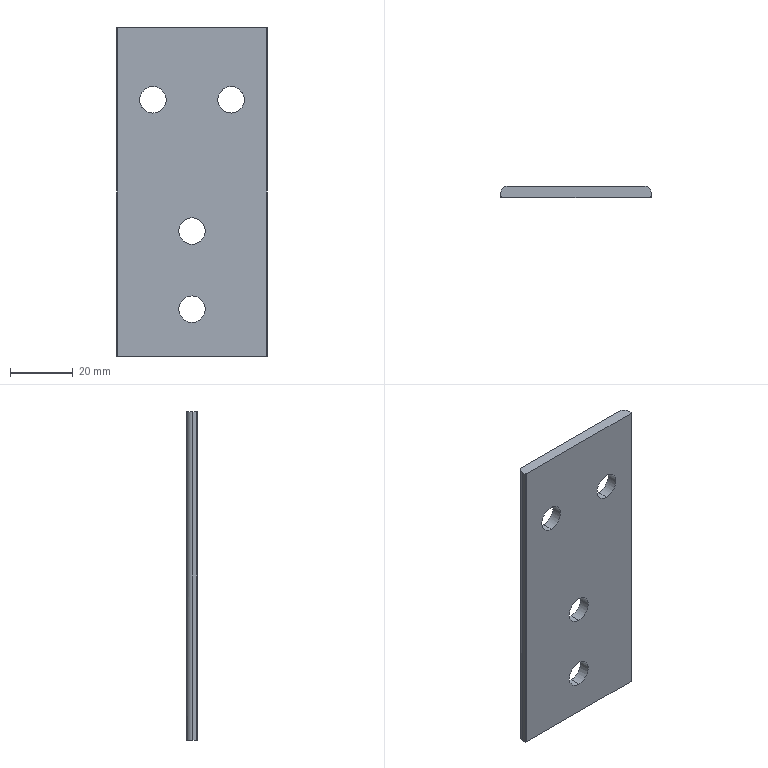Part | STEP file | 31E-01025QY13 | 1 solid | 18 faces | box 48 x 3.5 x 105 mm | volume 16661 mm3 | cylinder 12 | plane 6 | commonest cylinder face diameters 8.5 x8 0.6 x2 4 x2
STEP:
#1=CARTESIAN_POINT('',(0.,-1.75,10.75));
#2=VERTEX_POINT('',#1);
#3=CARTESIAN_POINT('',(0.,-1.75,19.25));
#4=VERTEX_POINT('',#3);
#5=CARTESIAN_POINT('',(0.,-1.75,15.));
#6=DIRECTION('',(0.,1.,0.));
#7=AXIS2_PLACEMENT_3D('',#5,#6,$);
#8=CIRCLE('',#7,4.25);
#9=EDGE_CURVE('',#2,#4,#8,.T.);
#10=ORIENTED_EDGE('',*,*,#9,.F.);
#11=CARTESIAN_POINT('',(0.,1.75,10.75));
#12=VERTEX_POINT('',#11);
#13=CARTESIAN_POINT('',(0.,-1.75,10.75));
#14=DIRECTION('',(0.,1.,0.));
#15=VECTOR('',#14,1.);
#16=LINE('',#13,#15);
#17=EDGE_CURVE('',#2,#12,#16,.T.);
#18=ORIENTED_EDGE('',*,*,#17,.T.);
#19=CARTESIAN_POINT('',(0.,1.75,19.25));
#20=VERTEX_POINT('',#19);
#21=CARTESIAN_POINT('',(0.,1.75,15.));
#22=DIRECTION('',(0.,1.,0.));
#23=AXIS2_PLACEMENT_3D('',#21,#22,$);
#24=CIRCLE('',#23,4.25);
#25=EDGE_CURVE('',#12,#20,#24,.T.);
#26=ORIENTED_EDGE('',*,*,#25,.T.);
#27=CARTESIAN_POINT('',(0.,-1.75,19.25));
#28=DIRECTION('',(0.,1.,0.));
#29=VECTOR('',#28,1.);
#30=LINE('',#27,#29);
#31=EDGE_CURVE('',#4,#20,#30,.T.);
#32=ORIENTED_EDGE('',*,*,#31,.F.);
#33=EDGE_LOOP('',(#10,#18,#26,#32));
#34=FACE_OUTER_BOUND('',#33,.T.);
#35=CARTESIAN_POINT('',(0.,-1.75,15.));
#36=DIRECTION('',(0.,1.,0.));
#37=DIRECTION('',(0.,0.,-1.));
#38=AXIS2_PLACEMENT_3D('',#35,#36,#37);
#39=CYLINDRICAL_SURFACE('',#38,4.25);
#40=ADVANCED_FACE('',(#34),#39,.F.);
#41=CARTESIAN_POINT('',(-23.7,-1.75,105.));
#42=VERTEX_POINT('',#41);
#43=CARTESIAN_POINT('',(23.7,-1.75,105.));
#44=VERTEX_POINT('',#43);
#45=CARTESIAN_POINT('',(0.,-1.75,105.));
#46=DIRECTION('',(1.,0.,0.));
#47=VECTOR('',#46,1.);
#48=LINE('',#45,#47);
#49=EDGE_CURVE('',#42,#44,#48,.T.);
#50=ORIENTED_EDGE('',*,*,#49,.F.);
#51=CARTESIAN_POINT('',(-23.7,-1.75,0.));
#52=VERTEX_POINT('',#51);
#53=CARTESIAN_POINT('',(-23.7,-1.75,52.5));
#54=DIRECTION('',(0.,0.,-1.));
#55=VECTOR('',#54,1.);
#56=LINE('',#53,#55);
#57=EDGE_CURVE('',#42,#52,#56,.T.);
#58=ORIENTED_EDGE('',*,*,#57,.T.);
#59=CARTESIAN_POINT('',(23.7,-1.75,0.));
#60=VERTEX_POINT('',#59);
#61=CARTESIAN_POINT('',(0.,-1.75,0.));
#62=DIRECTION('',(1.,0.,0.));
#63=VECTOR('',#62,1.);
#64=LINE('',#61,#63);
#65=EDGE_CURVE('',#52,#60,#64,.T.);
#66=ORIENTED_EDGE('',*,*,#65,.T.);
#67=CARTESIAN_POINT('',(23.7,-1.75,52.5));
#68=DIRECTION('',(0.,0.,1.));
#69=VECTOR('',#68,1.);
#70=LINE('',#67,#69);
#71=EDGE_CURVE('',#60,#44,#70,.T.);
#72=ORIENTED_EDGE('',*,*,#71,.T.);
#73=EDGE_LOOP('',(#50,#58,#66,#72));
#74=FACE_OUTER_BOUND('',#73,.T.);
#75=CARTESIAN_POINT('',(0.,-1.75,15.));
#76=DIRECTION('',(0.,1.,0.));
#77=AXIS2_PLACEMENT_3D('',#75,#76,$);
#78=CIRCLE('',#77,4.25);
#79=EDGE_CURVE('',#4,#2,#78,.T.);
#80=ORIENTED_EDGE('',*,*,#79,.T.);
#81=ORIENTED_EDGE('',*,*,#9,.T.);
#82=EDGE_LOOP('',(#80,#81));
#83=FACE_BOUND('',#82,.T.);
#84=CARTESIAN_POINT('',(0.,-1.75,44.25));
#85=VERTEX_POINT('',#84);
#86=CARTESIAN_POINT('',(0.,-1.75,35.75));
#87=VERTEX_POINT('',#86);
#88=CARTESIAN_POINT('',(0.,-1.75,40.));
#89=DIRECTION('',(0.,1.,0.));
#90=AXIS2_PLACEMENT_3D('',#88,#89,$);
#91=CIRCLE('',#90,4.25);
#92=EDGE_CURVE('',#85,#87,#91,.T.);
#93=ORIENTED_EDGE('',*,*,#92,.T.);
#94=CARTESIAN_POINT('',(0.,-1.75,40.));
#95=DIRECTION('',(0.,1.,0.));
#96=AXIS2_PLACEMENT_3D('',#94,#95,$);
#97=CIRCLE('',#96,4.25);
#98=EDGE_CURVE('',#87,#85,#97,.T.);
#99=ORIENTED_EDGE('',*,*,#98,.T.);
#100=EDGE_LOOP('',(#93,#99));
#101=FACE_BOUND('',#100,.T.);
#102=CARTESIAN_POINT('',(12.5,-1.75,86.25));
#103=VERTEX_POINT('',#102);
#104=CARTESIAN_POINT('',(12.5,-1.75,77.75));
#105=VERTEX_POINT('',#104);
#106=CARTESIAN_POINT('',(12.5,-1.75,82.));
#107=DIRECTION('',(0.,1.,0.));
#108=AXIS2_PLACEMENT_3D('',#106,#107,$);
#109=CIRCLE('',#108,4.25);
#110=EDGE_CURVE('',#103,#105,#109,.T.);
#111=ORIENTED_EDGE('',*,*,#110,.T.);
#112=CARTESIAN_POINT('',(12.5,-1.75,82.));
#113=DIRECTION('',(0.,1.,0.));
#114=AXIS2_PLACEMENT_3D('',#112,#113,$);
#115=CIRCLE('',#114,4.25);
#116=EDGE_CURVE('',#105,#103,#115,.T.);
#117=ORIENTED_EDGE('',*,*,#116,.T.);
#118=EDGE_LOOP('',(#111,#117));
#119=FACE_BOUND('',#118,.T.);
#120=CARTESIAN_POINT('',(-12.5,-1.75,86.25));
#121=VERTEX_POINT('',#120);
#122=CARTESIAN_POINT('',(-12.5,-1.75,77.75));
#123=VERTEX_POINT('',#122);
#124=CARTESIAN_POINT('',(-12.5,-1.75,82.));
#125=DIRECTION('',(0.,1.,0.));
#126=AXIS2_PLACEMENT_3D('',#124,#125,$);
#127=CIRCLE('',#126,4.25);
#128=EDGE_CURVE('',#121,#123,#127,.T.);
#129=ORIENTED_EDGE('',*,*,#128,.T.);
#130=CARTESIAN_POINT('',(-12.5,-1.75,82.));
#131=DIRECTION('',(0.,1.,0.));
#132=AXIS2_PLACEMENT_3D('',#130,#131,$);
#133=CIRCLE('',#132,4.25);
#134=EDGE_CURVE('',#123,#121,#133,.T.);
#135=ORIENTED_EDGE('',*,*,#134,.T.);
#136=EDGE_LOOP('',(#129,#135));
#137=FACE_BOUND('',#136,.T.);
#138=CARTESIAN_POINT('',(-24.,-1.75,105.));
#139=DIRECTION('',(0.,1.,0.));
#140=DIRECTION('',(0.,0.,1.));
#141=AXIS2_PLACEMENT_3D('',#138,#139,#140);
#142=PLANE('',#141);
#143=ADVANCED_FACE('',(#74,#83,#101,#119,#137),#142,.F.);
#144=ORIENTED_EDGE('',*,*,#17,.F.);
#145=ORIENTED_EDGE('',*,*,#79,.F.);
#146=ORIENTED_EDGE('',*,*,#31,.T.);
#147=CARTESIAN_POINT('',(0.,1.75,15.));
#148=DIRECTION('',(0.,1.,0.));
#149=AXIS2_PLACEMENT_3D('',#147,#148,$);
#150=CIRCLE('',#149,4.25);
#151=EDGE_CURVE('',#20,#12,#150,.T.);
#152=ORIENTED_EDGE('',*,*,#151,.T.);
#153=EDGE_LOOP('',(#144,#145,#146,#152));
#154=FACE_OUTER_BOUND('',#153,.T.);
#155=CARTESIAN_POINT('',(0.,-1.75,15.));
#156=DIRECTION('',(0.,1.,0.));
#157=DIRECTION('',(0.,0.,1.));
#158=AXIS2_PLACEMENT_3D('',#155,#156,#157);
#159=CYLINDRICAL_SURFACE('',#158,4.25);
#160=ADVANCED_FACE('',(#154),#159,.F.);
#161=CARTESIAN_POINT('',(22.,1.75,0.));
#162=VERTEX_POINT('',#161);
#163=CARTESIAN_POINT('',(-22.,1.75,0.));
#164=VERTEX_POINT('',#163);
#165=CARTESIAN_POINT('',(0.,1.75,0.));
#166=DIRECTION('',(-1.,0.,0.));
#167=VECTOR('',#166,1.);
#168=LINE('',#165,#167);
#169=EDGE_CURVE('',#162,#164,#168,.T.);
#170=ORIENTED_EDGE('',*,*,#169,.T.);
#171=CARTESIAN_POINT('',(-22.,1.75,105.));
#172=VERTEX_POINT('',#171);
#173=CARTESIAN_POINT('',(-22.,1.75,52.5));
#174=DIRECTION('',(0.,0.,1.));
#175=VECTOR('',#174,1.);
#176=LINE('',#173,#175);
#177=EDGE_CURVE('',#164,#172,#176,.T.);
#178=ORIENTED_EDGE('',*,*,#177,.T.);
#179=CARTESIAN_POINT('',(22.,1.75,105.));
#180=VERTEX_POINT('',#179);
#181=CARTESIAN_POINT('',(0.,1.75,105.));
#182=DIRECTION('',(-1.,0.,0.));
#183=VECTOR('',#182,1.);
#184=LINE('',#181,#183);
#185=EDGE_CURVE('',#180,#172,#184,.T.);
#186=ORIENTED_EDGE('',*,*,#185,.F.);
#187=CARTESIAN_POINT('',(22.,1.75,52.5));
#188=DIRECTION('',(0.,0.,-1.));
#189=VECTOR('',#188,1.);
#190=LINE('',#187,#189);
#191=EDGE_CURVE('',#180,#162,#190,.T.);
#192=ORIENTED_EDGE('',*,*,#191,.T.);
#193=EDGE_LOOP('',(#170,#178,#186,#192));
#194=FACE_OUTER_BOUND('',#193,.T.);
#195=ORIENTED_EDGE('',*,*,#151,.F.);
#196=ORIENTED_EDGE('',*,*,#25,.F.);
#197=EDGE_LOOP('',(#195,#196));
#198=FACE_BOUND('',#197,.T.);
#199=CARTESIAN_POINT('',(0.,1.75,44.25));
#200=VERTEX_POINT('',#199);
#201=CARTESIAN_POINT('',(0.,1.75,35.75));
#202=VERTEX_POINT('',#201);
#203=CARTESIAN_POINT('',(0.,1.75,44.25));
#204=CARTESIAN_POINT('',(0.404,1.75,44.25));
#205=CARTESIAN_POINT('',(0.808,1.75,44.202));
#206=CARTESIAN_POINT('',(1.204,1.75,44.106));
#207=CARTESIAN_POINT('',(1.967,1.75,43.822));
#208=CARTESIAN_POINT('',(2.641,1.75,43.367));
#209=CARTESIAN_POINT('',(2.95,1.75,43.1));
#210=CARTESIAN_POINT('',(3.497,1.75,42.498));
#211=CARTESIAN_POINT('',(3.889,1.75,41.785));
#212=CARTESIAN_POINT('',(4.041,1.75,41.407));
#213=CARTESIAN_POINT('',(4.253,1.75,40.621));
#214=CARTESIAN_POINT('',(4.275,1.75,39.808));
#215=CARTESIAN_POINT('',(4.237,1.75,39.402));
#216=CARTESIAN_POINT('',(4.066,1.75,38.606));
#217=CARTESIAN_POINT('',(3.713,1.75,37.873));
#218=CARTESIAN_POINT('',(3.493,1.75,37.529));
#219=CARTESIAN_POINT('',(2.977,1.75,36.9));
#220=CARTESIAN_POINT('',(2.328,1.75,36.41));
#221=CARTESIAN_POINT('',(1.976,1.75,36.204));
#222=CARTESIAN_POINT('',(1.374,1.75,35.944));
#223=CARTESIAN_POINT('',(0.7377,1.75,35.804));
#224=CARTESIAN_POINT('',(0.4929,1.75,35.768));
#225=CARTESIAN_POINT('',(0.2465,1.75,35.75));
#226=CARTESIAN_POINT('',(0.,1.75,35.75));
#227=B_SPLINE_CURVE_WITH_KNOTS('',5,(#203,#204,#205,#206,#207,#208,#209,#210,#211,#212,#213,#214,#215,#216,#217,#218,#219,#220,#221,#222,#223,#224,#225,#226),.UNSPECIFIED.,.F.,.U.,(6,3,3,3,3,3,3,6),(0.,2.857,5.713,8.57,11.426,14.283,17.139,18.882),.UNSPECIFIED.);
#228=EDGE_CURVE('',#200,#202,#227,.T.);
#229=ORIENTED_EDGE('',*,*,#228,.F.);
#230=CARTESIAN_POINT('',(0.,1.75,35.75));
#231=CARTESIAN_POINT('',(-0.404,1.75,35.75));
#232=CARTESIAN_POINT('',(-0.808,1.75,35.798));
#233=CARTESIAN_POINT('',(-1.204,1.75,35.894));
#234=CARTESIAN_POINT('',(-1.967,1.75,36.178));
#235=CARTESIAN_POINT('',(-2.641,1.75,36.633));
#236=CARTESIAN_POINT('',(-2.95,1.75,36.9));
#237=CARTESIAN_POINT('',(-3.497,1.75,37.502));
#238=CARTESIAN_POINT('',(-3.889,1.75,38.215));
#239=CARTESIAN_POINT('',(-4.041,1.75,38.593));
#240=CARTESIAN_POINT('',(-4.253,1.75,39.379));
#241=CARTESIAN_POINT('',(-4.275,1.75,40.192));
#242=CARTESIAN_POINT('',(-4.237,1.75,40.598));
#243=CARTESIAN_POINT('',(-4.066,1.75,41.394));
#244=CARTESIAN_POINT('',(-3.713,1.75,42.127));
#245=CARTESIAN_POINT('',(-3.493,1.75,42.471));
#246=CARTESIAN_POINT('',(-2.977,1.75,43.1));
#247=CARTESIAN_POINT('',(-2.328,1.75,43.59));
#248=CARTESIAN_POINT('',(-1.976,1.75,43.796));
#249=CARTESIAN_POINT('',(-1.374,1.75,44.056));
#250=CARTESIAN_POINT('',(-0.7377,1.75,44.196));
#251=CARTESIAN_POINT('',(-0.4929,1.75,44.232));
#252=CARTESIAN_POINT('',(-0.2465,1.75,44.25));
#253=CARTESIAN_POINT('',(0.,1.75,44.25));
#254=B_SPLINE_CURVE_WITH_KNOTS('',5,(#230,#231,#232,#233,#234,#235,#236,#237,#238,#239,#240,#241,#242,#243,#244,#245,#246,#247,#248,#249,#250,#251,#252,#253),.UNSPECIFIED.,.F.,.U.,(6,3,3,3,3,3,3,6),(0.,2.857,5.713,8.57,11.426,14.283,17.139,18.882),.UNSPECIFIED.);
#255=EDGE_CURVE('',#202,#200,#254,.T.);
#256=ORIENTED_EDGE('',*,*,#255,.F.);
#257=EDGE_LOOP('',(#229,#256));
#258=FACE_BOUND('',#257,.T.);
#259=CARTESIAN_POINT('',(12.5,1.75,86.25));
#260=VERTEX_POINT('',#259);
#261=CARTESIAN_POINT('',(12.5,1.75,77.75));
#262=VERTEX_POINT('',#261);
#263=CARTESIAN_POINT('',(12.5,1.75,86.25));
#264=CARTESIAN_POINT('',(12.904,1.75,86.25));
#265=CARTESIAN_POINT('',(13.308,1.75,86.202));
#266=CARTESIAN_POINT('',(13.704,1.75,86.106));
#267=CARTESIAN_POINT('',(14.467,1.75,85.822));
#268=CARTESIAN_POINT('',(15.141,1.75,85.367));
#269=CARTESIAN_POINT('',(15.45,1.75,85.1));
#270=CARTESIAN_POINT('',(15.997,1.75,84.498));
#271=CARTESIAN_POINT('',(16.389,1.75,83.785));
#272=CARTESIAN_POINT('',(16.541,1.75,83.407));
#273=CARTESIAN_POINT('',(16.753,1.75,82.621));
#274=CARTESIAN_POINT('',(16.775,1.75,81.808));
#275=CARTESIAN_POINT('',(16.737,1.75,81.402));
#276=CARTESIAN_POINT('',(16.566,1.75,80.606));
#277=CARTESIAN_POINT('',(16.213,1.75,79.873));
#278=CARTESIAN_POINT('',(15.993,1.75,79.529));
#279=CARTESIAN_POINT('',(15.477,1.75,78.9));
#280=CARTESIAN_POINT('',(14.828,1.75,78.41));
#281=CARTESIAN_POINT('',(14.476,1.75,78.204));
#282=CARTESIAN_POINT('',(13.874,1.75,77.944));
#283=CARTESIAN_POINT('',(13.238,1.75,77.804));
#284=CARTESIAN_POINT('',(12.993,1.75,77.768));
#285=CARTESIAN_POINT('',(12.746,1.75,77.75));
#286=CARTESIAN_POINT('',(12.5,1.75,77.75));
#287=B_SPLINE_CURVE_WITH_KNOTS('',5,(#263,#264,#265,#266,#267,#268,#269,#270,#271,#272,#273,#274,#275,#276,#277,#278,#279,#280,#281,#282,#283,#284,#285,#286),.UNSPECIFIED.,.F.,.U.,(6,3,3,3,3,3,3,6),(0.,2.857,5.713,8.57,11.426,14.283,17.139,18.882),.UNSPECIFIED.);
#288=EDGE_CURVE('',#260,#262,#287,.T.);
#289=ORIENTED_EDGE('',*,*,#288,.F.);
#290=CARTESIAN_POINT('',(12.5,1.75,77.75));
#291=CARTESIAN_POINT('',(12.096,1.75,77.75));
#292=CARTESIAN_POINT('',(11.692,1.75,77.798));
#293=CARTESIAN_POINT('',(11.296,1.75,77.894));
#294=CARTESIAN_POINT('',(10.533,1.75,78.178));
#295=CARTESIAN_POINT('',(9.859,1.75,78.633));
#296=CARTESIAN_POINT('',(9.55,1.75,78.9));
#297=CARTESIAN_POINT('',(9.003,1.75,79.502));
#298=CARTESIAN_POINT('',(8.611,1.75,80.215));
#299=CARTESIAN_POINT('',(8.459,1.75,80.593));
#300=CARTESIAN_POINT('',(8.247,1.75,81.379));
#301=CARTESIAN_POINT('',(8.225,1.75,82.192));
#302=CARTESIAN_POINT('',(8.263,1.75,82.598));
#303=CARTESIAN_POINT('',(8.434,1.75,83.394));
#304=CARTESIAN_POINT('',(8.787,1.75,84.127));
#305=CARTESIAN_POINT('',(9.007,1.75,84.471));
#306=CARTESIAN_POINT('',(9.523,1.75,85.1));
#307=CARTESIAN_POINT('',(10.172,1.75,85.59));
#308=CARTESIAN_POINT('',(10.524,1.75,85.796));
#309=CARTESIAN_POINT('',(11.126,1.75,86.056));
#310=CARTESIAN_POINT('',(11.762,1.75,86.196));
#311=CARTESIAN_POINT('',(12.007,1.75,86.232));
#312=CARTESIAN_POINT('',(12.254,1.75,86.25));
#313=CARTESIAN_POINT('',(12.5,1.75,86.25));
#314=B_SPLINE_CURVE_WITH_KNOTS('',5,(#290,#291,#292,#293,#294,#295,#296,#297,#298,#299,#300,#301,#302,#303,#304,#305,#306,#307,#308,#309,#310,#311,#312,#313),.UNSPECIFIED.,.F.,.U.,(6,3,3,3,3,3,3,6),(0.,2.857,5.713,8.57,11.426,14.283,17.139,18.882),.UNSPECIFIED.);
#315=EDGE_CURVE('',#262,#260,#314,.T.);
#316=ORIENTED_EDGE('',*,*,#315,.F.);
#317=EDGE_LOOP('',(#289,#316));
#318=FACE_BOUND('',#317,.T.);
#319=CARTESIAN_POINT('',(-12.5,1.75,86.25));
#320=VERTEX_POINT('',#319);
#321=CARTESIAN_POINT('',(-12.5,1.75,77.75));
#322=VERTEX_POINT('',#321);
#323=CARTESIAN_POINT('',(-12.5,1.75,86.25));
#324=CARTESIAN_POINT('',(-12.096,1.75,86.25));
#325=CARTESIAN_POINT('',(-11.692,1.75,86.202));
#326=CARTESIAN_POINT('',(-11.296,1.75,86.106));
#327=CARTESIAN_POINT('',(-10.533,1.75,85.822));
#328=CARTESIAN_POINT('',(-9.859,1.75,85.367));
#329=CARTESIAN_POINT('',(-9.55,1.75,85.1));
#330=CARTESIAN_POINT('',(-9.003,1.75,84.498));
#331=CARTESIAN_POINT('',(-8.611,1.75,83.785));
#332=CARTESIAN_POINT('',(-8.459,1.75,83.407));
#333=CARTESIAN_POINT('',(-8.247,1.75,82.621));
#334=CARTESIAN_POINT('',(-8.225,1.75,81.808));
#335=CARTESIAN_POINT('',(-8.263,1.75,81.402));
#336=CARTESIAN_POINT('',(-8.434,1.75,80.606));
#337=CARTESIAN_POINT('',(-8.787,1.75,79.873));
#338=CARTESIAN_POINT('',(-9.007,1.75,79.529));
#339=CARTESIAN_POINT('',(-9.523,1.75,78.9));
#340=CARTESIAN_POINT('',(-10.172,1.75,78.41));
#341=CARTESIAN_POINT('',(-10.524,1.75,78.204));
#342=CARTESIAN_POINT('',(-11.126,1.75,77.944));
#343=CARTESIAN_POINT('',(-11.762,1.75,77.804));
#344=CARTESIAN_POINT('',(-12.007,1.75,77.768));
#345=CARTESIAN_POINT('',(-12.254,1.75,77.75));
#346=CARTESIAN_POINT('',(-12.5,1.75,77.75));
#347=B_SPLINE_CURVE_WITH_KNOTS('',5,(#323,#324,#325,#326,#327,#328,#329,#330,#331,#332,#333,#334,#335,#336,#337,#338,#339,#340,#341,#342,#343,#344,#345,#346),.UNSPECIFIED.,.F.,.U.,(6,3,3,3,3,3,3,6),(0.,2.857,5.713,8.57,11.426,14.283,17.139,18.882),.UNSPECIFIED.);
#348=EDGE_CURVE('',#320,#322,#347,.T.);
#349=ORIENTED_EDGE('',*,*,#348,.F.);
#350=CARTESIAN_POINT('',(-12.5,1.75,77.75));
#351=CARTESIAN_POINT('',(-12.904,1.75,77.75));
#352=CARTESIAN_POINT('',(-13.308,1.75,77.798));
#353=CARTESIAN_POINT('',(-13.704,1.75,77.894));
#354=CARTESIAN_POINT('',(-14.467,1.75,78.178));
#355=CARTESIAN_POINT('',(-15.141,1.75,78.633));
#356=CARTESIAN_POINT('',(-15.45,1.75,78.9));
#357=CARTESIAN_POINT('',(-15.997,1.75,79.502));
#358=CARTESIAN_POINT('',(-16.389,1.75,80.215));
#359=CARTESIAN_POINT('',(-16.541,1.75,80.593));
#360=CARTESIAN_POINT('',(-16.753,1.75,81.379));
#361=CARTESIAN_POINT('',(-16.775,1.75,82.192));
#362=CARTESIAN_POINT('',(-16.737,1.75,82.598));
#363=CARTESIAN_POINT('',(-16.566,1.75,83.394));
#364=CARTESIAN_POINT('',(-16.213,1.75,84.127));
#365=CARTESIAN_POINT('',(-15.993,1.75,84.471));
#366=CARTESIAN_POINT('',(-15.477,1.75,85.1));
#367=CARTESIAN_POINT('',(-14.828,1.75,85.59));
#368=CARTESIAN_POINT('',(-14.476,1.75,85.796));
#369=CARTESIAN_POINT('',(-13.874,1.75,86.056));
#370=CARTESIAN_POINT('',(-13.238,1.75,86.196));
#371=CARTESIAN_POINT('',(-12.993,1.75,86.232));
#372=CARTESIAN_POINT('',(-12.746,1.75,86.25));
#373=CARTESIAN_POINT('',(-12.5,1.75,86.25));
#374=B_SPLINE_CURVE_WITH_KNOTS('',5,(#350,#351,#352,#353,#354,#355,#356,#357,#358,#359,#360,#361,#362,#363,#364,#365,#366,#367,#368,#369,#370,#371,#372,#373),.UNSPECIFIED.,.F.,.U.,(6,3,3,3,3,3,3,6),(0.,2.857,5.713,8.57,11.426,14.283,17.139,18.882),.UNSPECIFIED.);
#375=EDGE_CURVE('',#322,#320,#374,.T.);
#376=ORIENTED_EDGE('',*,*,#375,.F.);
#377=EDGE_LOOP('',(#349,#376));
#378=FACE_BOUND('',#377,.T.);
#379=CARTESIAN_POINT('',(-24.,1.75,105.));
#380=DIRECTION('',(0.,-1.,0.));
#381=DIRECTION('',(0.,0.,-1.));
#382=AXIS2_PLACEMENT_3D('',#379,#380,#381);
#383=PLANE('',#382);
#384=ADVANCED_FACE('',(#194,#198,#258,#318,#378),#383,.F.);
#385=CARTESIAN_POINT('',(-24.,-0.25,105.));
#386=VERTEX_POINT('',#385);
#387=CARTESIAN_POINT('',(-24.,-1.45,105.));
#388=VERTEX_POINT('',#387);
#389=CARTESIAN_POINT('',(-24.,-0.85,105.));
#390=DIRECTION('',(0.,-1.,0.));
#391=VECTOR('',#390,1.);
#392=LINE('',#389,#391);
#393=EDGE_CURVE('',#386,#388,#392,.T.);
#394=ORIENTED_EDGE('',*,*,#393,.T.);
#395=CARTESIAN_POINT('',(-23.7,-1.45,105.));
#396=DIRECTION('',(0.,0.,1.));
#397=AXIS2_PLACEMENT_3D('',#395,#396,$);
#398=CIRCLE('',#397,0.3);
#399=EDGE_CURVE('',#388,#42,#398,.T.);
#400=ORIENTED_EDGE('',*,*,#399,.T.);
#401=ORIENTED_EDGE('',*,*,#49,.T.);
#402=CARTESIAN_POINT('',(24.,-1.45,105.));
#403=VERTEX_POINT('',#402);
#404=CARTESIAN_POINT('',(23.7,-1.45,105.));
#405=DIRECTION('',(0.,0.,1.));
#406=AXIS2_PLACEMENT_3D('',#404,#405,$);
#407=CIRCLE('',#406,0.3);
#408=EDGE_CURVE('',#44,#403,#407,.T.);
#409=ORIENTED_EDGE('',*,*,#408,.T.);
#410=CARTESIAN_POINT('',(24.,-0.25,105.));
#411=VERTEX_POINT('',#410);
#412=CARTESIAN_POINT('',(24.,-0.85,105.));
#413=DIRECTION('',(0.,1.,0.));
#414=VECTOR('',#413,1.);
#415=LINE('',#412,#414);
#416=EDGE_CURVE('',#403,#411,#415,.T.);
#417=ORIENTED_EDGE('',*,*,#416,.T.);
#418=CARTESIAN_POINT('',(22.,-0.25,105.));
#419=DIRECTION('',(0.,0.,1.));
#420=AXIS2_PLACEMENT_3D('',#418,#419,$);
#421=CIRCLE('',#420,2.);
#422=EDGE_CURVE('',#411,#180,#421,.T.);
#423=ORIENTED_EDGE('',*,*,#422,.T.);
#424=ORIENTED_EDGE('',*,*,#185,.T.);
#425=CARTESIAN_POINT('',(-22.,-0.25,105.));
#426=DIRECTION('',(0.,0.,1.));
#427=AXIS2_PLACEMENT_3D('',#425,#426,$);
#428=CIRCLE('',#427,2.);
#429=EDGE_CURVE('',#172,#386,#428,.T.);
#430=ORIENTED_EDGE('',*,*,#429,.T.);
#431=EDGE_LOOP('',(#394,#400,#401,#409,#417,#423,#424,#430));
#432=FACE_OUTER_BOUND('',#431,.T.);
#433=CARTESIAN_POINT('',(24.,-1.75,105.));
#434=DIRECTION('',(0.,0.,1.));
#435=DIRECTION('',(1.,0.,0.));
#436=AXIS2_PLACEMENT_3D('',#433,#434,#435);
#437=PLANE('',#436);
#438=ADVANCED_FACE('',(#432),#437,.T.);
#439=ORIENTED_EDGE('',*,*,#399,.F.);
#440=CARTESIAN_POINT('',(-24.,-1.45,0.));
#441=VERTEX_POINT('',#440);
#442=CARTESIAN_POINT('',(-24.,-1.45,105.));
#443=DIRECTION('',(0.,0.,-1.));
#444=VECTOR('',#443,1.);
#445=LINE('',#442,#444);
#446=EDGE_CURVE('',#441,#388,#445,.F.);
#447=ORIENTED_EDGE('',*,*,#446,.F.);
#448=CARTESIAN_POINT('',(-23.7,-1.45,0.));
#449=DIRECTION('',(0.,0.,-1.));
#450=AXIS2_PLACEMENT_3D('',#448,#449,$);
#451=CIRCLE('',#450,0.3);
#452=EDGE_CURVE('',#52,#441,#451,.T.);
#453=ORIENTED_EDGE('',*,*,#452,.F.);
#454=ORIENTED_EDGE('',*,*,#57,.F.);
#455=EDGE_LOOP('',(#439,#447,#453,#454));
#456=FACE_OUTER_BOUND('',#455,.T.);
#457=CARTESIAN_POINT('',(-23.7,-1.45,105.));
#458=DIRECTION('',(0.,0.,-1.));
#459=DIRECTION('',(1.,0.,0.));
#460=AXIS2_PLACEMENT_3D('',#457,#458,#459);
#461=CYLINDRICAL_SURFACE('',#460,0.3);
#462=ADVANCED_FACE('',(#456),#461,.T.);
#463=ORIENTED_EDGE('',*,*,#65,.F.);
#464=ORIENTED_EDGE('',*,*,#452,.T.);
#465=CARTESIAN_POINT('',(-24.,-0.25,0.));
#466=VERTEX_POINT('',#465);
#467=CARTESIAN_POINT('',(-24.,-0.85,0.));
#468=DIRECTION('',(0.,-1.,0.));
#469=VECTOR('',#468,1.);
#470=LINE('',#467,#469);
#471=EDGE_CURVE('',#466,#441,#470,.T.);
#472=ORIENTED_EDGE('',*,*,#471,.F.);
#473=CARTESIAN_POINT('',(-24.,-0.25,0.));
#474=CARTESIAN_POINT('',(-24.,-0.04216,0.));
#475=CARTESIAN_POINT('',(-23.973,0.1657,0.));
#476=CARTESIAN_POINT('',(-23.919,0.3689,0.));
#477=CARTESIAN_POINT('',(-23.759,0.7565,0.));
#478=CARTESIAN_POINT('',(-23.506,1.091,0.));
#479=CARTESIAN_POINT('',(-23.358,1.24,0.));
#480=CARTESIAN_POINT('',(-23.027,1.497,0.));
#481=CARTESIAN_POINT('',(-22.642,1.661,0.));
#482=CARTESIAN_POINT('',(-22.439,1.718,0.));
#483=CARTESIAN_POINT('',(-22.227,1.748,0.));
#484=CARTESIAN_POINT('',(-22.014,1.75,0.));
#485=CARTESIAN_POINT('',(-22.01,1.75,0.));
#486=CARTESIAN_POINT('',(-22.005,1.75,0.));
#487=CARTESIAN_POINT('',(-22.,1.75,0.));
#488=B_SPLINE_CURVE_WITH_KNOTS('',5,(#473,#474,#475,#476,#477,#478,#479,#480,#481,#482,#483,#484,#485,#486,#487),.UNSPECIFIED.,.F.,.U.,(6,3,3,3,6),(0.,1.47,2.939,4.409,4.443),.UNSPECIFIED.);
#489=EDGE_CURVE('',#466,#164,#488,.T.);
#490=ORIENTED_EDGE('',*,*,#489,.T.);
#491=ORIENTED_EDGE('',*,*,#169,.F.);
#492=CARTESIAN_POINT('',(24.,-0.25,0.));
#493=VERTEX_POINT('',#492);
#494=CARTESIAN_POINT('',(22.,1.75,0.));
#495=CARTESIAN_POINT('',(22.208,1.75,0.));
#496=CARTESIAN_POINT('',(22.416,1.723,0.));
#497=CARTESIAN_POINT('',(22.619,1.669,0.));
#498=CARTESIAN_POINT('',(23.006,1.509,0.));
#499=CARTESIAN_POINT('',(23.341,1.256,0.));
#500=CARTESIAN_POINT('',(23.49,1.108,0.));
#501=CARTESIAN_POINT('',(23.747,0.7775,0.));
#502=CARTESIAN_POINT('',(23.911,0.3918,0.));
#503=CARTESIAN_POINT('',(23.968,0.1892,0.));
#504=CARTESIAN_POINT('',(23.998,-0.02304,0.));
#505=CARTESIAN_POINT('',(24.,-0.2357,0.));
#506=CARTESIAN_POINT('',(24.,-0.2404,0.));
#507=CARTESIAN_POINT('',(24.,-0.2452,0.));
#508=CARTESIAN_POINT('',(24.,-0.25,0.));
#509=B_SPLINE_CURVE_WITH_KNOTS('',5,(#494,#495,#496,#497,#498,#499,#500,#501,#502,#503,#504,#505,#506,#507,#508),.UNSPECIFIED.,.F.,.U.,(6,3,3,3,6),(0.,1.47,2.939,4.409,4.443),.UNSPECIFIED.);
#510=EDGE_CURVE('',#162,#493,#509,.T.);
#511=ORIENTED_EDGE('',*,*,#510,.T.);
#512=CARTESIAN_POINT('',(24.,-1.45,0.));
#513=VERTEX_POINT('',#512);
#514=CARTESIAN_POINT('',(24.,-0.85,0.));
#515=DIRECTION('',(0.,1.,0.));
#516=VECTOR('',#515,1.);
#517=LINE('',#514,#516);
#518=EDGE_CURVE('',#513,#493,#517,.T.);
#519=ORIENTED_EDGE('',*,*,#518,.F.);
#520=CARTESIAN_POINT('',(24.,-1.45,0.));
#521=CARTESIAN_POINT('',(24.,-1.487,0.));
#522=CARTESIAN_POINT('',(23.994,-1.525,0.));
#523=CARTESIAN_POINT('',(23.982,-1.562,0.));
#524=CARTESIAN_POINT('',(23.947,-1.63,0.));
#525=CARTESIAN_POINT('',(23.894,-1.683,0.));
#526=CARTESIAN_POINT('',(23.862,-1.707,0.));
#527=CARTESIAN_POINT('',(23.811,-1.732,0.));
#528=CARTESIAN_POINT('',(23.756,-1.746,0.));
#529=CARTESIAN_POINT('',(23.738,-1.749,0.));
#530=CARTESIAN_POINT('',(23.719,-1.75,0.));
#531=CARTESIAN_POINT('',(23.7,-1.75,0.));
#532=B_SPLINE_CURVE_WITH_KNOTS('',5,(#520,#521,#522,#523,#524,#525,#526,#527,#528,#529,#530,#531),.UNSPECIFIED.,.F.,.U.,(6,3,3,6),(0.,0.2644,0.5288,0.6618),.UNSPECIFIED.);
#533=EDGE_CURVE('',#513,#60,#532,.T.);
#534=ORIENTED_EDGE('',*,*,#533,.T.);
#535=EDGE_LOOP('',(#463,#464,#472,#490,#491,#511,#519,#534));
#536=FACE_OUTER_BOUND('',#535,.T.);
#537=CARTESIAN_POINT('',(24.,-1.75,0.));
#538=DIRECTION('',(0.,0.,1.));
#539=DIRECTION('',(1.,0.,0.));
#540=AXIS2_PLACEMENT_3D('',#537,#538,#539);
#541=PLANE('',#540);
#542=ADVANCED_FACE('',(#536),#541,.F.);
#543=ORIENTED_EDGE('',*,*,#408,.F.);
#544=ORIENTED_EDGE('',*,*,#71,.F.);
#545=ORIENTED_EDGE('',*,*,#533,.F.);
#546=CARTESIAN_POINT('',(24.,-1.45,105.));
#547=DIRECTION('',(0.,0.,-1.));
#548=VECTOR('',#547,1.);
#549=LINE('',#546,#548);
#550=EDGE_CURVE('',#403,#513,#549,.T.);
#551=ORIENTED_EDGE('',*,*,#550,.F.);
#552=EDGE_LOOP('',(#543,#544,#545,#551));
#553=FACE_OUTER_BOUND('',#552,.T.);
#554=CARTESIAN_POINT('',(23.7,-1.45,105.));
#555=DIRECTION('',(0.,0.,-1.));
#556=DIRECTION('',(1.,0.,0.));
#557=AXIS2_PLACEMENT_3D('',#554,#555,#556);
#558=CYLINDRICAL_SURFACE('',#557,0.3);
#559=ADVANCED_FACE('',(#553),#558,.T.);
#560=CARTESIAN_POINT('',(0.,-1.75,35.75));
#561=DIRECTION('',(0.,1.,0.));
#562=VECTOR('',#561,1.);
#563=LINE('',#560,#562);
#564=EDGE_CURVE('',#87,#202,#563,.T.);
#565=ORIENTED_EDGE('',*,*,#564,.F.);
#566=ORIENTED_EDGE('',*,*,#92,.F.);
#567=CARTESIAN_POINT('',(0.,-1.75,44.25));
#568=DIRECTION('',(0.,1.,0.));
#569=VECTOR('',#568,1.);
#570=LINE('',#567,#569);
#571=EDGE_CURVE('',#85,#200,#570,.T.);
#572=ORIENTED_EDGE('',*,*,#571,.T.);
#573=ORIENTED_EDGE('',*,*,#228,.T.);
#574=EDGE_LOOP('',(#565,#566,#572,#573));
#575=FACE_OUTER_BOUND('',#574,.T.);
#576=CARTESIAN_POINT('',(0.,-1.75,40.));
#577=DIRECTION('',(0.,1.,0.));
#578=DIRECTION('',(0.,0.,1.));
#579=AXIS2_PLACEMENT_3D('',#576,#577,#578);
#580=CYLINDRICAL_SURFACE('',#579,4.25);
#581=ADVANCED_FACE('',(#575),#580,.F.);
#582=ORIENTED_EDGE('',*,*,#98,.F.);
#583=ORIENTED_EDGE('',*,*,#564,.T.);
#584=ORIENTED_EDGE('',*,*,#255,.T.);
#585=ORIENTED_EDGE('',*,*,#571,.F.);
#586=EDGE_LOOP('',(#582,#583,#584,#585));
#587=FACE_OUTER_BOUND('',#586,.T.);
#588=CARTESIAN_POINT('',(0.,-1.75,40.));
#589=DIRECTION('',(0.,1.,0.));
#590=DIRECTION('',(0.,0.,-1.));
#591=AXIS2_PLACEMENT_3D('',#588,#589,#590);
#592=CYLINDRICAL_SURFACE('',#591,4.25);
#593=ADVANCED_FACE('',(#587),#592,.F.);
#594=CARTESIAN_POINT('',(12.5,-1.75,77.75));
#595=DIRECTION('',(0.,1.,0.));
#596=VECTOR('',#595,1.);
#597=LINE('',#594,#596);
#598=EDGE_CURVE('',#105,#262,#597,.T.);
#599=ORIENTED_EDGE('',*,*,#598,.F.);
#600=ORIENTED_EDGE('',*,*,#110,.F.);
#601=CARTESIAN_POINT('',(12.5,-1.75,86.25));
#602=DIRECTION('',(0.,1.,0.));
#603=VECTOR('',#602,1.);
#604=LINE('',#601,#603);
#605=EDGE_CURVE('',#103,#260,#604,.T.);
#606=ORIENTED_EDGE('',*,*,#605,.T.);
#607=ORIENTED_EDGE('',*,*,#288,.T.);
#608=EDGE_LOOP('',(#599,#600,#606,#607));
#609=FACE_OUTER_BOUND('',#608,.T.);
#610=CARTESIAN_POINT('',(12.5,-1.75,82.));
#611=DIRECTION('',(0.,1.,0.));
#612=DIRECTION('',(0.,0.,1.));
#613=AXIS2_PLACEMENT_3D('',#610,#611,#612);
#614=CYLINDRICAL_SURFACE('',#613,4.25);
#615=ADVANCED_FACE('',(#609),#614,.F.);
#616=ORIENTED_EDGE('',*,*,#116,.F.);
#617=ORIENTED_EDGE('',*,*,#598,.T.);
#618=ORIENTED_EDGE('',*,*,#315,.T.);
#619=ORIENTED_EDGE('',*,*,#605,.F.);
#620=EDGE_LOOP('',(#616,#617,#618,#619));
#621=FACE_OUTER_BOUND('',#620,.T.);
#622=CARTESIAN_POINT('',(12.5,-1.75,82.));
#623=DIRECTION('',(0.,1.,0.));
#624=DIRECTION('',(0.,0.,-1.));
#625=AXIS2_PLACEMENT_3D('',#622,#623,#624);
#626=CYLINDRICAL_SURFACE('',#625,4.25);
#627=ADVANCED_FACE('',(#621),#626,.F.);
#628=CARTESIAN_POINT('',(-12.5,-1.75,77.75));
#629=DIRECTION('',(0.,1.,0.));
#630=VECTOR('',#629,1.);
#631=LINE('',#628,#630);
#632=EDGE_CURVE('',#123,#322,#631,.T.);
#633=ORIENTED_EDGE('',*,*,#632,.F.);
#634=ORIENTED_EDGE('',*,*,#128,.F.);
#635=CARTESIAN_POINT('',(-12.5,-1.75,86.25));
#636=DIRECTION('',(0.,1.,0.));
#637=VECTOR('',#636,1.);
#638=LINE('',#635,#637);
#639=EDGE_CURVE('',#121,#320,#638,.T.);
#640=ORIENTED_EDGE('',*,*,#639,.T.);
#641=ORIENTED_EDGE('',*,*,#348,.T.);
#642=EDGE_LOOP('',(#633,#634,#640,#641));
#643=FACE_OUTER_BOUND('',#642,.T.);
#644=CARTESIAN_POINT('',(-12.5,-1.75,82.));
#645=DIRECTION('',(0.,1.,0.));
#646=DIRECTION('',(0.,0.,1.));
#647=AXIS2_PLACEMENT_3D('',#644,#645,#646);
#648=CYLINDRICAL_SURFACE('',#647,4.25);
#649=ADVANCED_FACE('',(#643),#648,.F.);
#650=ORIENTED_EDGE('',*,*,#134,.F.);
#651=ORIENTED_EDGE('',*,*,#632,.T.);
#652=ORIENTED_EDGE('',*,*,#375,.T.);
#653=ORIENTED_EDGE('',*,*,#639,.F.);
#654=EDGE_LOOP('',(#650,#651,#652,#653));
#655=FACE_OUTER_BOUND('',#654,.T.);
#656=CARTESIAN_POINT('',(-12.5,-1.75,82.));
#657=DIRECTION('',(0.,1.,0.));
#658=DIRECTION('',(0.,0.,-1.));
#659=AXIS2_PLACEMENT_3D('',#656,#657,#658);
#660=CYLINDRICAL_SURFACE('',#659,4.25);
#661=ADVANCED_FACE('',(#655),#660,.F.);
#662=ORIENTED_EDGE('',*,*,#429,.F.);
#663=ORIENTED_EDGE('',*,*,#177,.F.);
#664=ORIENTED_EDGE('',*,*,#489,.F.);
#665=CARTESIAN_POINT('',(-24.,-0.25,105.));
#666=DIRECTION('',(0.,0.,-1.));
#667=VECTOR('',#666,1.);
#668=LINE('',#665,#667);
#669=EDGE_CURVE('',#386,#466,#668,.T.);
#670=ORIENTED_EDGE('',*,*,#669,.F.);
#671=EDGE_LOOP('',(#662,#663,#664,#670));
#672=FACE_OUTER_BOUND('',#671,.T.);
#673=CARTESIAN_POINT('',(-22.,-0.25,105.));
#674=DIRECTION('',(0.,0.,-1.));
#675=DIRECTION('',(-1.,0.,0.));
#676=AXIS2_PLACEMENT_3D('',#673,#674,#675);
#677=CYLINDRICAL_SURFACE('',#676,2.);
#678=ADVANCED_FACE('',(#672),#677,.T.);
#679=ORIENTED_EDGE('',*,*,#422,.F.);
#680=CARTESIAN_POINT('',(24.,-0.25,105.));
#681=DIRECTION('',(0.,0.,-1.));
#682=VECTOR('',#681,1.);
#683=LINE('',#680,#682);
#684=EDGE_CURVE('',#493,#411,#683,.F.);
#685=ORIENTED_EDGE('',*,*,#684,.F.);
#686=ORIENTED_EDGE('',*,*,#510,.F.);
#687=ORIENTED_EDGE('',*,*,#191,.F.);
#688=EDGE_LOOP('',(#679,#685,#686,#687));
#689=FACE_OUTER_BOUND('',#688,.T.);
#690=CARTESIAN_POINT('',(22.,-0.25,105.));
#691=DIRECTION('',(0.,0.,-1.));
#692=DIRECTION('',(-1.,0.,0.));
#693=AXIS2_PLACEMENT_3D('',#690,#691,#692);
#694=CYLINDRICAL_SURFACE('',#693,2.);
#695=ADVANCED_FACE('',(#689),#694,.T.);
#696=ORIENTED_EDGE('',*,*,#471,.T.);
#697=ORIENTED_EDGE('',*,*,#446,.T.);
#698=ORIENTED_EDGE('',*,*,#393,.F.);
#699=ORIENTED_EDGE('',*,*,#669,.T.);
#700=EDGE_LOOP('',(#696,#697,#698,#699));
#701=FACE_OUTER_BOUND('',#700,.T.);
#702=CARTESIAN_POINT('',(-24.,1.75,105.));
#703=DIRECTION('',(1.,0.,0.));
#704=DIRECTION('',(0.,0.,-1.));
#705=AXIS2_PLACEMENT_3D('',#702,#703,#704);
#706=PLANE('',#705);
#707=ADVANCED_FACE('',(#701),#706,.F.);
#708=ORIENTED_EDGE('',*,*,#416,.F.);
#709=ORIENTED_EDGE('',*,*,#550,.T.);
#710=ORIENTED_EDGE('',*,*,#518,.T.);
#711=ORIENTED_EDGE('',*,*,#684,.T.);
#712=EDGE_LOOP('',(#708,#709,#710,#711));
#713=FACE_OUTER_BOUND('',#712,.T.);
#714=CARTESIAN_POINT('',(24.,1.75,105.));
#715=DIRECTION('',(-1.,0.,0.));
#716=DIRECTION('',(0.,-1.,0.));
#717=AXIS2_PLACEMENT_3D('',#714,#715,#716);
#718=PLANE('',#717);
#719=ADVANCED_FACE('',(#713),#718,.F.);
#720=CLOSED_SHELL('',(#40,#143,#160,#384,#438,#462,#542,#559,#581,#593,#615,#627,#649,#661,#678,#695,#707,#719));
#721=MANIFOLD_SOLID_BREP('',#720);
#722=(LENGTH_UNIT()NAMED_UNIT(*)SI_UNIT(.MILLI.,.METRE.));
#723=UNCERTAINTY_MEASURE_WITH_UNIT(LENGTH_MEASURE(0.005),#722,'','');
#724=(NAMED_UNIT(*)PLANE_ANGLE_UNIT()SI_UNIT($,.RADIAN.));
#725=(NAMED_UNIT(*)SI_UNIT($,.STERADIAN.)SOLID_ANGLE_UNIT());
#726=(GEOMETRIC_REPRESENTATION_CONTEXT(3)GLOBAL_UNCERTAINTY_ASSIGNED_CONTEXT((#723))GLOBAL_UNIT_ASSIGNED_CONTEXT((#722,#724,#725))REPRESENTATION_CONTEXT('',''));
#727=ADVANCED_BREP_SHAPE_REPRESENTATION('',(#721),#726);